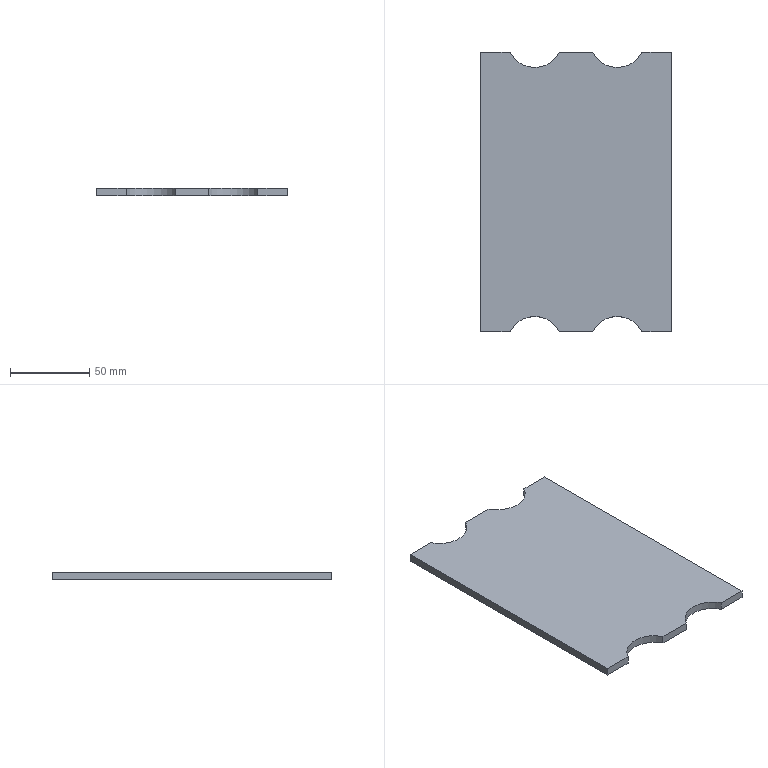Part | SolidWorks | features BaseBody 1 | 1 solid | 14 faces | box 120 x 176 x 5 mm | volume 101377 mm3 | plane 10 | cylinder 4 | commonest cylinder face diameters 35 x4
STEP:
#1=CARTESIAN_POINT('',(172.899,88.,322.));
#2=VERTEX_POINT('',#1);
#3=CARTESIAN_POINT('',(172.899,-88.,322.));
#4=VERTEX_POINT('',#3);
#5=CARTESIAN_POINT('',(172.899,88.,322.));
#6=DIRECTION('',(0.,-1.,0.));
#7=VECTOR('',#6,1000.);
#8=LINE('',#5,#7);
#9=EDGE_CURVE('',#2,#4,#8,.T.);
#10=ORIENTED_EDGE('',*,*,#9,.F.);
#11=CARTESIAN_POINT('',(191.335,88.,322.));
#12=VERTEX_POINT('',#11);
#13=CARTESIAN_POINT('',(191.335,88.,322.));
#14=DIRECTION('',(-1.,0.,0.));
#15=VECTOR('',#14,1000.);
#16=LINE('',#13,#15);
#17=EDGE_CURVE('',#12,#2,#16,.T.);
#18=ORIENTED_EDGE('',*,*,#17,.F.);
#19=CARTESIAN_POINT('',(222.464,88.,322.));
#20=VERTEX_POINT('',#19);
#21=CARTESIAN_POINT('',(206.899,96.,322.));
#22=DIRECTION('',(0.,0.,-1.));
#23=DIRECTION('',(0.8894,-0.4571,0.));
#24=AXIS2_PLACEMENT_3D('',#21,#22,#23);
#25=CIRCLE('',#24,17.5);
#26=EDGE_CURVE('',#20,#12,#25,.T.);
#27=ORIENTED_EDGE('',*,*,#26,.F.);
#28=CARTESIAN_POINT('',(243.335,88.,322.));
#29=VERTEX_POINT('',#28);
#30=CARTESIAN_POINT('',(243.335,88.,322.));
#31=DIRECTION('',(-1.,0.,0.));
#32=VECTOR('',#31,1000.);
#33=LINE('',#30,#32);
#34=EDGE_CURVE('',#29,#20,#33,.T.);
#35=ORIENTED_EDGE('',*,*,#34,.F.);
#36=CARTESIAN_POINT('',(274.464,88.,322.));
#37=VERTEX_POINT('',#36);
#38=CARTESIAN_POINT('',(258.899,96.,322.));
#39=DIRECTION('',(0.,0.,-1.));
#40=DIRECTION('',(0.8894,-0.4571,0.));
#41=AXIS2_PLACEMENT_3D('',#38,#39,#40);
#42=CIRCLE('',#41,17.5);
#43=EDGE_CURVE('',#37,#29,#42,.T.);
#44=ORIENTED_EDGE('',*,*,#43,.F.);
#45=CARTESIAN_POINT('',(292.899,88.,322.));
#46=VERTEX_POINT('',#45);
#47=CARTESIAN_POINT('',(292.899,88.,322.));
#48=DIRECTION('',(-1.,0.,0.));
#49=VECTOR('',#48,1000.);
#50=LINE('',#47,#49);
#51=EDGE_CURVE('',#46,#37,#50,.T.);
#52=ORIENTED_EDGE('',*,*,#51,.F.);
#53=CARTESIAN_POINT('',(292.899,-88.,322.));
#54=VERTEX_POINT('',#53);
#55=CARTESIAN_POINT('',(292.899,-88.,322.));
#56=DIRECTION('',(0.,1.,0.));
#57=VECTOR('',#56,1000.);
#58=LINE('',#55,#57);
#59=EDGE_CURVE('',#54,#46,#58,.T.);
#60=ORIENTED_EDGE('',*,*,#59,.F.);
#61=CARTESIAN_POINT('',(274.464,-88.,322.));
#62=VERTEX_POINT('',#61);
#63=CARTESIAN_POINT('',(274.464,-88.,322.));
#64=DIRECTION('',(1.,0.,0.));
#65=VECTOR('',#64,1000.);
#66=LINE('',#63,#65);
#67=EDGE_CURVE('',#62,#54,#66,.T.);
#68=ORIENTED_EDGE('',*,*,#67,.F.);
#69=CARTESIAN_POINT('',(243.335,-88.,322.));
#70=VERTEX_POINT('',#69);
#71=CARTESIAN_POINT('',(258.899,-96.,322.));
#72=DIRECTION('',(0.,0.,-1.));
#73=DIRECTION('',(-0.8894,0.4571,0.));
#74=AXIS2_PLACEMENT_3D('',#71,#72,#73);
#75=CIRCLE('',#74,17.5);
#76=EDGE_CURVE('',#70,#62,#75,.T.);
#77=ORIENTED_EDGE('',*,*,#76,.F.);
#78=CARTESIAN_POINT('',(222.464,-88.,322.));
#79=VERTEX_POINT('',#78);
#80=CARTESIAN_POINT('',(222.464,-88.,322.));
#81=DIRECTION('',(1.,0.,0.));
#82=VECTOR('',#81,1000.);
#83=LINE('',#80,#82);
#84=EDGE_CURVE('',#79,#70,#83,.T.);
#85=ORIENTED_EDGE('',*,*,#84,.F.);
#86=CARTESIAN_POINT('',(191.335,-88.,322.));
#87=VERTEX_POINT('',#86);
#88=CARTESIAN_POINT('',(206.899,-96.,322.));
#89=DIRECTION('',(0.,0.,-1.));
#90=DIRECTION('',(-0.8894,0.4571,0.));
#91=AXIS2_PLACEMENT_3D('',#88,#89,#90);
#92=CIRCLE('',#91,17.5);
#93=EDGE_CURVE('',#87,#79,#92,.T.);
#94=ORIENTED_EDGE('',*,*,#93,.F.);
#95=CARTESIAN_POINT('',(172.899,-88.,322.));
#96=DIRECTION('',(1.,0.,0.));
#97=VECTOR('',#96,1000.);
#98=LINE('',#95,#97);
#99=EDGE_CURVE('',#4,#87,#98,.T.);
#100=ORIENTED_EDGE('',*,*,#99,.F.);
#101=EDGE_LOOP('',(#10,#18,#27,#35,#44,#52,#60,#68,#77,#85,#94,#100));
#102=FACE_OUTER_BOUND('',#101,.T.);
#103=CARTESIAN_POINT('',(206.899,-96.,322.));
#104=DIRECTION('',(0.,0.,-1.));
#105=DIRECTION('',(0.,-1.,0.));
#106=AXIS2_PLACEMENT_3D('',#103,#104,#105);
#107=PLANE('',#106);
#108=ADVANCED_FACE('',(#102),#107,.T.);
#109=CARTESIAN_POINT('',(172.899,-88.,327.));
#110=VERTEX_POINT('',#109);
#111=CARTESIAN_POINT('',(172.899,88.,327.));
#112=VERTEX_POINT('',#111);
#113=CARTESIAN_POINT('',(172.899,-88.,327.));
#114=DIRECTION('',(0.,1.,0.));
#115=VECTOR('',#114,1000.);
#116=LINE('',#113,#115);
#117=EDGE_CURVE('',#110,#112,#116,.T.);
#118=ORIENTED_EDGE('',*,*,#117,.F.);
#119=CARTESIAN_POINT('',(191.335,-88.,327.));
#120=VERTEX_POINT('',#119);
#121=CARTESIAN_POINT('',(191.335,-88.,327.));
#122=DIRECTION('',(-1.,0.,0.));
#123=VECTOR('',#122,1000.);
#124=LINE('',#121,#123);
#125=EDGE_CURVE('',#120,#110,#124,.T.);
#126=ORIENTED_EDGE('',*,*,#125,.F.);
#127=CARTESIAN_POINT('',(222.464,-88.,327.));
#128=VERTEX_POINT('',#127);
#129=CARTESIAN_POINT('',(206.899,-96.,327.));
#130=DIRECTION('',(0.,0.,1.));
#131=DIRECTION('',(0.8894,0.4571,0.));
#132=AXIS2_PLACEMENT_3D('',#129,#130,#131);
#133=CIRCLE('',#132,17.5);
#134=EDGE_CURVE('',#128,#120,#133,.T.);
#135=ORIENTED_EDGE('',*,*,#134,.F.);
#136=CARTESIAN_POINT('',(243.335,-88.,327.));
#137=VERTEX_POINT('',#136);
#138=CARTESIAN_POINT('',(243.335,-88.,327.));
#139=DIRECTION('',(-1.,0.,0.));
#140=VECTOR('',#139,1000.);
#141=LINE('',#138,#140);
#142=EDGE_CURVE('',#137,#128,#141,.T.);
#143=ORIENTED_EDGE('',*,*,#142,.F.);
#144=CARTESIAN_POINT('',(274.464,-88.,327.));
#145=VERTEX_POINT('',#144);
#146=CARTESIAN_POINT('',(258.899,-96.,327.));
#147=DIRECTION('',(0.,0.,1.));
#148=DIRECTION('',(0.8894,0.4571,0.));
#149=AXIS2_PLACEMENT_3D('',#146,#147,#148);
#150=CIRCLE('',#149,17.5);
#151=EDGE_CURVE('',#145,#137,#150,.T.);
#152=ORIENTED_EDGE('',*,*,#151,.F.);
#153=CARTESIAN_POINT('',(292.899,-88.,327.));
#154=VERTEX_POINT('',#153);
#155=CARTESIAN_POINT('',(292.899,-88.,327.));
#156=DIRECTION('',(-1.,0.,0.));
#157=VECTOR('',#156,1000.);
#158=LINE('',#155,#157);
#159=EDGE_CURVE('',#154,#145,#158,.T.);
#160=ORIENTED_EDGE('',*,*,#159,.F.);
#161=CARTESIAN_POINT('',(292.899,88.,327.));
#162=VERTEX_POINT('',#161);
#163=CARTESIAN_POINT('',(292.899,88.,327.));
#164=DIRECTION('',(0.,-1.,0.));
#165=VECTOR('',#164,1000.);
#166=LINE('',#163,#165);
#167=EDGE_CURVE('',#162,#154,#166,.T.);
#168=ORIENTED_EDGE('',*,*,#167,.F.);
#169=CARTESIAN_POINT('',(274.464,88.,327.));
#170=VERTEX_POINT('',#169);
#171=CARTESIAN_POINT('',(274.464,88.,327.));
#172=DIRECTION('',(1.,0.,0.));
#173=VECTOR('',#172,1000.);
#174=LINE('',#171,#173);
#175=EDGE_CURVE('',#170,#162,#174,.T.);
#176=ORIENTED_EDGE('',*,*,#175,.F.);
#177=CARTESIAN_POINT('',(243.335,88.,327.));
#178=VERTEX_POINT('',#177);
#179=CARTESIAN_POINT('',(258.899,96.,327.));
#180=DIRECTION('',(0.,0.,1.));
#181=DIRECTION('',(-0.8894,-0.4571,0.));
#182=AXIS2_PLACEMENT_3D('',#179,#180,#181);
#183=CIRCLE('',#182,17.5);
#184=EDGE_CURVE('',#178,#170,#183,.T.);
#185=ORIENTED_EDGE('',*,*,#184,.F.);
#186=CARTESIAN_POINT('',(222.464,88.,327.));
#187=VERTEX_POINT('',#186);
#188=CARTESIAN_POINT('',(222.464,88.,327.));
#189=DIRECTION('',(1.,0.,0.));
#190=VECTOR('',#189,1000.);
#191=LINE('',#188,#190);
#192=EDGE_CURVE('',#187,#178,#191,.T.);
#193=ORIENTED_EDGE('',*,*,#192,.F.);
#194=CARTESIAN_POINT('',(191.335,88.,327.));
#195=VERTEX_POINT('',#194);
#196=CARTESIAN_POINT('',(206.899,96.,327.));
#197=DIRECTION('',(0.,0.,1.));
#198=DIRECTION('',(-0.8894,-0.4571,0.));
#199=AXIS2_PLACEMENT_3D('',#196,#197,#198);
#200=CIRCLE('',#199,17.5);
#201=EDGE_CURVE('',#195,#187,#200,.T.);
#202=ORIENTED_EDGE('',*,*,#201,.F.);
#203=CARTESIAN_POINT('',(172.899,88.,327.));
#204=DIRECTION('',(1.,0.,0.));
#205=VECTOR('',#204,1000.);
#206=LINE('',#203,#205);
#207=EDGE_CURVE('',#112,#195,#206,.T.);
#208=ORIENTED_EDGE('',*,*,#207,.F.);
#209=EDGE_LOOP('',(#118,#126,#135,#143,#152,#160,#168,#176,#185,#193,#202,#208));
#210=FACE_OUTER_BOUND('',#209,.T.);
#211=CARTESIAN_POINT('',(206.899,-96.,327.));
#212=DIRECTION('',(0.,0.,1.));
#213=DIRECTION('',(1.,0.,0.));
#214=AXIS2_PLACEMENT_3D('',#211,#212,#213);
#215=PLANE('',#214);
#216=ADVANCED_FACE('',(#210),#215,.T.);
#217=ORIENTED_EDGE('',*,*,#17,.T.);
#218=CARTESIAN_POINT('',(172.899,88.,327.));
#219=DIRECTION('',(0.,0.,-1.));
#220=VECTOR('',#219,1000.);
#221=LINE('',#218,#220);
#222=EDGE_CURVE('',#112,#2,#221,.T.);
#223=ORIENTED_EDGE('',*,*,#222,.F.);
#224=ORIENTED_EDGE('',*,*,#207,.T.);
#225=CARTESIAN_POINT('',(191.335,88.,322.));
#226=DIRECTION('',(0.,0.,1.));
#227=VECTOR('',#226,1000.);
#228=LINE('',#225,#227);
#229=EDGE_CURVE('',#12,#195,#228,.T.);
#230=ORIENTED_EDGE('',*,*,#229,.F.);
#231=EDGE_LOOP('',(#217,#223,#224,#230));
#232=FACE_OUTER_BOUND('',#231,.T.);
#233=CARTESIAN_POINT('',(191.335,88.,327.));
#234=DIRECTION('',(0.,1.,0.));
#235=DIRECTION('',(1.,0.,0.));
#236=AXIS2_PLACEMENT_3D('',#233,#234,#235);
#237=PLANE('',#236);
#238=ADVANCED_FACE('',(#232),#237,.T.);
#239=ORIENTED_EDGE('',*,*,#26,.T.);
#240=ORIENTED_EDGE('',*,*,#229,.T.);
#241=ORIENTED_EDGE('',*,*,#201,.T.);
#242=CARTESIAN_POINT('',(222.464,88.,322.));
#243=DIRECTION('',(0.,0.,1.));
#244=VECTOR('',#243,1000.);
#245=LINE('',#242,#244);
#246=EDGE_CURVE('',#20,#187,#245,.T.);
#247=ORIENTED_EDGE('',*,*,#246,.F.);
#248=EDGE_LOOP('',(#239,#240,#241,#247));
#249=FACE_OUTER_BOUND('',#248,.T.);
#250=CARTESIAN_POINT('',(206.899,96.,327.));
#251=DIRECTION('',(0.,0.,-1.));
#252=DIRECTION('',(-0.8894,0.4571,0.));
#253=AXIS2_PLACEMENT_3D('',#250,#251,#252);
#254=CYLINDRICAL_SURFACE('',#253,17.5);
#255=ADVANCED_FACE('',(#249),#254,.F.);
#256=ORIENTED_EDGE('',*,*,#34,.T.);
#257=ORIENTED_EDGE('',*,*,#246,.T.);
#258=ORIENTED_EDGE('',*,*,#192,.T.);
#259=CARTESIAN_POINT('',(243.335,88.,322.));
#260=DIRECTION('',(0.,0.,1.));
#261=VECTOR('',#260,1000.);
#262=LINE('',#259,#261);
#263=EDGE_CURVE('',#29,#178,#262,.T.);
#264=ORIENTED_EDGE('',*,*,#263,.F.);
#265=EDGE_LOOP('',(#256,#257,#258,#264));
#266=FACE_OUTER_BOUND('',#265,.T.);
#267=CARTESIAN_POINT('',(243.335,88.,327.));
#268=DIRECTION('',(0.,1.,0.));
#269=DIRECTION('',(1.,0.,0.));
#270=AXIS2_PLACEMENT_3D('',#267,#268,#269);
#271=PLANE('',#270);
#272=ADVANCED_FACE('',(#266),#271,.T.);
#273=ORIENTED_EDGE('',*,*,#43,.T.);
#274=ORIENTED_EDGE('',*,*,#263,.T.);
#275=ORIENTED_EDGE('',*,*,#184,.T.);
#276=CARTESIAN_POINT('',(274.464,88.,322.));
#277=DIRECTION('',(0.,0.,1.));
#278=VECTOR('',#277,1000.);
#279=LINE('',#276,#278);
#280=EDGE_CURVE('',#37,#170,#279,.T.);
#281=ORIENTED_EDGE('',*,*,#280,.F.);
#282=EDGE_LOOP('',(#273,#274,#275,#281));
#283=FACE_OUTER_BOUND('',#282,.T.);
#284=CARTESIAN_POINT('',(258.899,96.,327.));
#285=DIRECTION('',(0.,0.,-1.));
#286=DIRECTION('',(-0.8894,0.4571,0.));
#287=AXIS2_PLACEMENT_3D('',#284,#285,#286);
#288=CYLINDRICAL_SURFACE('',#287,17.5);
#289=ADVANCED_FACE('',(#283),#288,.F.);
#290=ORIENTED_EDGE('',*,*,#51,.T.);
#291=ORIENTED_EDGE('',*,*,#280,.T.);
#292=ORIENTED_EDGE('',*,*,#175,.T.);
#293=CARTESIAN_POINT('',(292.899,88.,322.));
#294=DIRECTION('',(0.,0.,1.));
#295=VECTOR('',#294,1000.);
#296=LINE('',#293,#295);
#297=EDGE_CURVE('',#46,#162,#296,.T.);
#298=ORIENTED_EDGE('',*,*,#297,.F.);
#299=EDGE_LOOP('',(#290,#291,#292,#298));
#300=FACE_OUTER_BOUND('',#299,.T.);
#301=CARTESIAN_POINT('',(292.899,88.,327.));
#302=DIRECTION('',(0.,1.,0.));
#303=DIRECTION('',(1.,0.,0.));
#304=AXIS2_PLACEMENT_3D('',#301,#302,#303);
#305=PLANE('',#304);
#306=ADVANCED_FACE('',(#300),#305,.T.);
#307=ORIENTED_EDGE('',*,*,#59,.T.);
#308=ORIENTED_EDGE('',*,*,#297,.T.);
#309=ORIENTED_EDGE('',*,*,#167,.T.);
#310=CARTESIAN_POINT('',(292.899,-88.,322.));
#311=DIRECTION('',(0.,0.,1.));
#312=VECTOR('',#311,1000.);
#313=LINE('',#310,#312);
#314=EDGE_CURVE('',#54,#154,#313,.T.);
#315=ORIENTED_EDGE('',*,*,#314,.F.);
#316=EDGE_LOOP('',(#307,#308,#309,#315));
#317=FACE_OUTER_BOUND('',#316,.T.);
#318=CARTESIAN_POINT('',(292.899,-88.,327.));
#319=DIRECTION('',(1.,0.,0.));
#320=DIRECTION('',(0.,1.,0.));
#321=AXIS2_PLACEMENT_3D('',#318,#319,#320);
#322=PLANE('',#321);
#323=ADVANCED_FACE('',(#317),#322,.T.);
#324=ORIENTED_EDGE('',*,*,#67,.T.);
#325=ORIENTED_EDGE('',*,*,#314,.T.);
#326=ORIENTED_EDGE('',*,*,#159,.T.);
#327=CARTESIAN_POINT('',(274.464,-88.,322.));
#328=DIRECTION('',(0.,0.,1.));
#329=VECTOR('',#328,1000.);
#330=LINE('',#327,#329);
#331=EDGE_CURVE('',#62,#145,#330,.T.);
#332=ORIENTED_EDGE('',*,*,#331,.F.);
#333=EDGE_LOOP('',(#324,#325,#326,#332));
#334=FACE_OUTER_BOUND('',#333,.T.);
#335=CARTESIAN_POINT('',(274.464,-88.,327.));
#336=DIRECTION('',(0.,-1.,0.));
#337=DIRECTION('',(0.,0.,-1.));
#338=AXIS2_PLACEMENT_3D('',#335,#336,#337);
#339=PLANE('',#338);
#340=ADVANCED_FACE('',(#334),#339,.T.);
#341=ORIENTED_EDGE('',*,*,#76,.T.);
#342=ORIENTED_EDGE('',*,*,#331,.T.);
#343=ORIENTED_EDGE('',*,*,#151,.T.);
#344=CARTESIAN_POINT('',(243.335,-88.,322.));
#345=DIRECTION('',(0.,0.,1.));
#346=VECTOR('',#345,1000.);
#347=LINE('',#344,#346);
#348=EDGE_CURVE('',#70,#137,#347,.T.);
#349=ORIENTED_EDGE('',*,*,#348,.F.);
#350=EDGE_LOOP('',(#341,#342,#343,#349));
#351=FACE_OUTER_BOUND('',#350,.T.);
#352=CARTESIAN_POINT('',(258.899,-96.,327.));
#353=DIRECTION('',(0.,0.,-1.));
#354=DIRECTION('',(0.8894,-0.4571,0.));
#355=AXIS2_PLACEMENT_3D('',#352,#353,#354);
#356=CYLINDRICAL_SURFACE('',#355,17.5);
#357=ADVANCED_FACE('',(#351),#356,.F.);
#358=ORIENTED_EDGE('',*,*,#84,.T.);
#359=ORIENTED_EDGE('',*,*,#348,.T.);
#360=ORIENTED_EDGE('',*,*,#142,.T.);
#361=CARTESIAN_POINT('',(222.464,-88.,322.));
#362=DIRECTION('',(0.,0.,1.));
#363=VECTOR('',#362,1000.);
#364=LINE('',#361,#363);
#365=EDGE_CURVE('',#79,#128,#364,.T.);
#366=ORIENTED_EDGE('',*,*,#365,.F.);
#367=EDGE_LOOP('',(#358,#359,#360,#366));
#368=FACE_OUTER_BOUND('',#367,.T.);
#369=CARTESIAN_POINT('',(222.464,-88.,327.));
#370=DIRECTION('',(0.,-1.,0.));
#371=DIRECTION('',(0.,0.,-1.));
#372=AXIS2_PLACEMENT_3D('',#369,#370,#371);
#373=PLANE('',#372);
#374=ADVANCED_FACE('',(#368),#373,.T.);
#375=ORIENTED_EDGE('',*,*,#93,.T.);
#376=ORIENTED_EDGE('',*,*,#365,.T.);
#377=ORIENTED_EDGE('',*,*,#134,.T.);
#378=CARTESIAN_POINT('',(191.335,-88.,322.));
#379=DIRECTION('',(0.,0.,1.));
#380=VECTOR('',#379,1000.);
#381=LINE('',#378,#380);
#382=EDGE_CURVE('',#87,#120,#381,.T.);
#383=ORIENTED_EDGE('',*,*,#382,.F.);
#384=EDGE_LOOP('',(#375,#376,#377,#383));
#385=FACE_OUTER_BOUND('',#384,.T.);
#386=CARTESIAN_POINT('',(206.899,-96.,327.));
#387=DIRECTION('',(0.,0.,-1.));
#388=DIRECTION('',(0.8894,-0.4571,0.));
#389=AXIS2_PLACEMENT_3D('',#386,#387,#388);
#390=CYLINDRICAL_SURFACE('',#389,17.5);
#391=ADVANCED_FACE('',(#385),#390,.F.);
#392=ORIENTED_EDGE('',*,*,#99,.T.);
#393=ORIENTED_EDGE('',*,*,#382,.T.);
#394=ORIENTED_EDGE('',*,*,#125,.T.);
#395=CARTESIAN_POINT('',(172.899,-88.,322.));
#396=DIRECTION('',(0.,0.,1.));
#397=VECTOR('',#396,1000.);
#398=LINE('',#395,#397);
#399=EDGE_CURVE('',#4,#110,#398,.T.);
#400=ORIENTED_EDGE('',*,*,#399,.F.);
#401=EDGE_LOOP('',(#392,#393,#394,#400));
#402=FACE_OUTER_BOUND('',#401,.T.);
#403=CARTESIAN_POINT('',(172.899,-88.,327.));
#404=DIRECTION('',(0.,-1.,0.));
#405=DIRECTION('',(0.,0.,-1.));
#406=AXIS2_PLACEMENT_3D('',#403,#404,#405);
#407=PLANE('',#406);
#408=ADVANCED_FACE('',(#402),#407,.T.);
#409=ORIENTED_EDGE('',*,*,#9,.T.);
#410=ORIENTED_EDGE('',*,*,#399,.T.);
#411=ORIENTED_EDGE('',*,*,#117,.T.);
#412=ORIENTED_EDGE('',*,*,#222,.T.);
#413=EDGE_LOOP('',(#409,#410,#411,#412));
#414=FACE_OUTER_BOUND('',#413,.T.);
#415=CARTESIAN_POINT('',(172.899,88.,327.));
#416=DIRECTION('',(-1.,0.,0.));
#417=DIRECTION('',(0.,0.,1.));
#418=AXIS2_PLACEMENT_3D('',#415,#416,#417);
#419=PLANE('',#418);
#420=ADVANCED_FACE('',(#414),#419,.T.);
#421=CLOSED_SHELL('',(#108,#216,#238,#255,#272,#289,#306,#323,#340,#357,#374,#391,#408,#420));
#422=MANIFOLD_SOLID_BREP('',#421);
#423=CARTESIAN_POINT('',(0.,0.,0.));
#424=DIRECTION('',(0.,0.,1.));
#425=DIRECTION('',(1.,0.,0.));
#426=AXIS2_PLACEMENT_3D('',#423,#424,#425);
#427=(LENGTH_UNIT()NAMED_UNIT(*)SI_UNIT(.MILLI.,.METRE.));
#428=UNCERTAINTY_MEASURE_WITH_UNIT(LENGTH_MEASURE(0.00001),#427,'','');
#429=(NAMED_UNIT(*)PLANE_ANGLE_UNIT()SI_UNIT($,.RADIAN.));
#430=(NAMED_UNIT(*)SI_UNIT($,.STERADIAN.)SOLID_ANGLE_UNIT());
#431=(GEOMETRIC_REPRESENTATION_CONTEXT(3)GLOBAL_UNCERTAINTY_ASSIGNED_CONTEXT((#428))GLOBAL_UNIT_ASSIGNED_CONTEXT((#427,#429,#430))REPRESENTATION_CONTEXT('',''));
#432=ADVANCED_BREP_SHAPE_REPRESENTATION('',(#422,#426),#431);